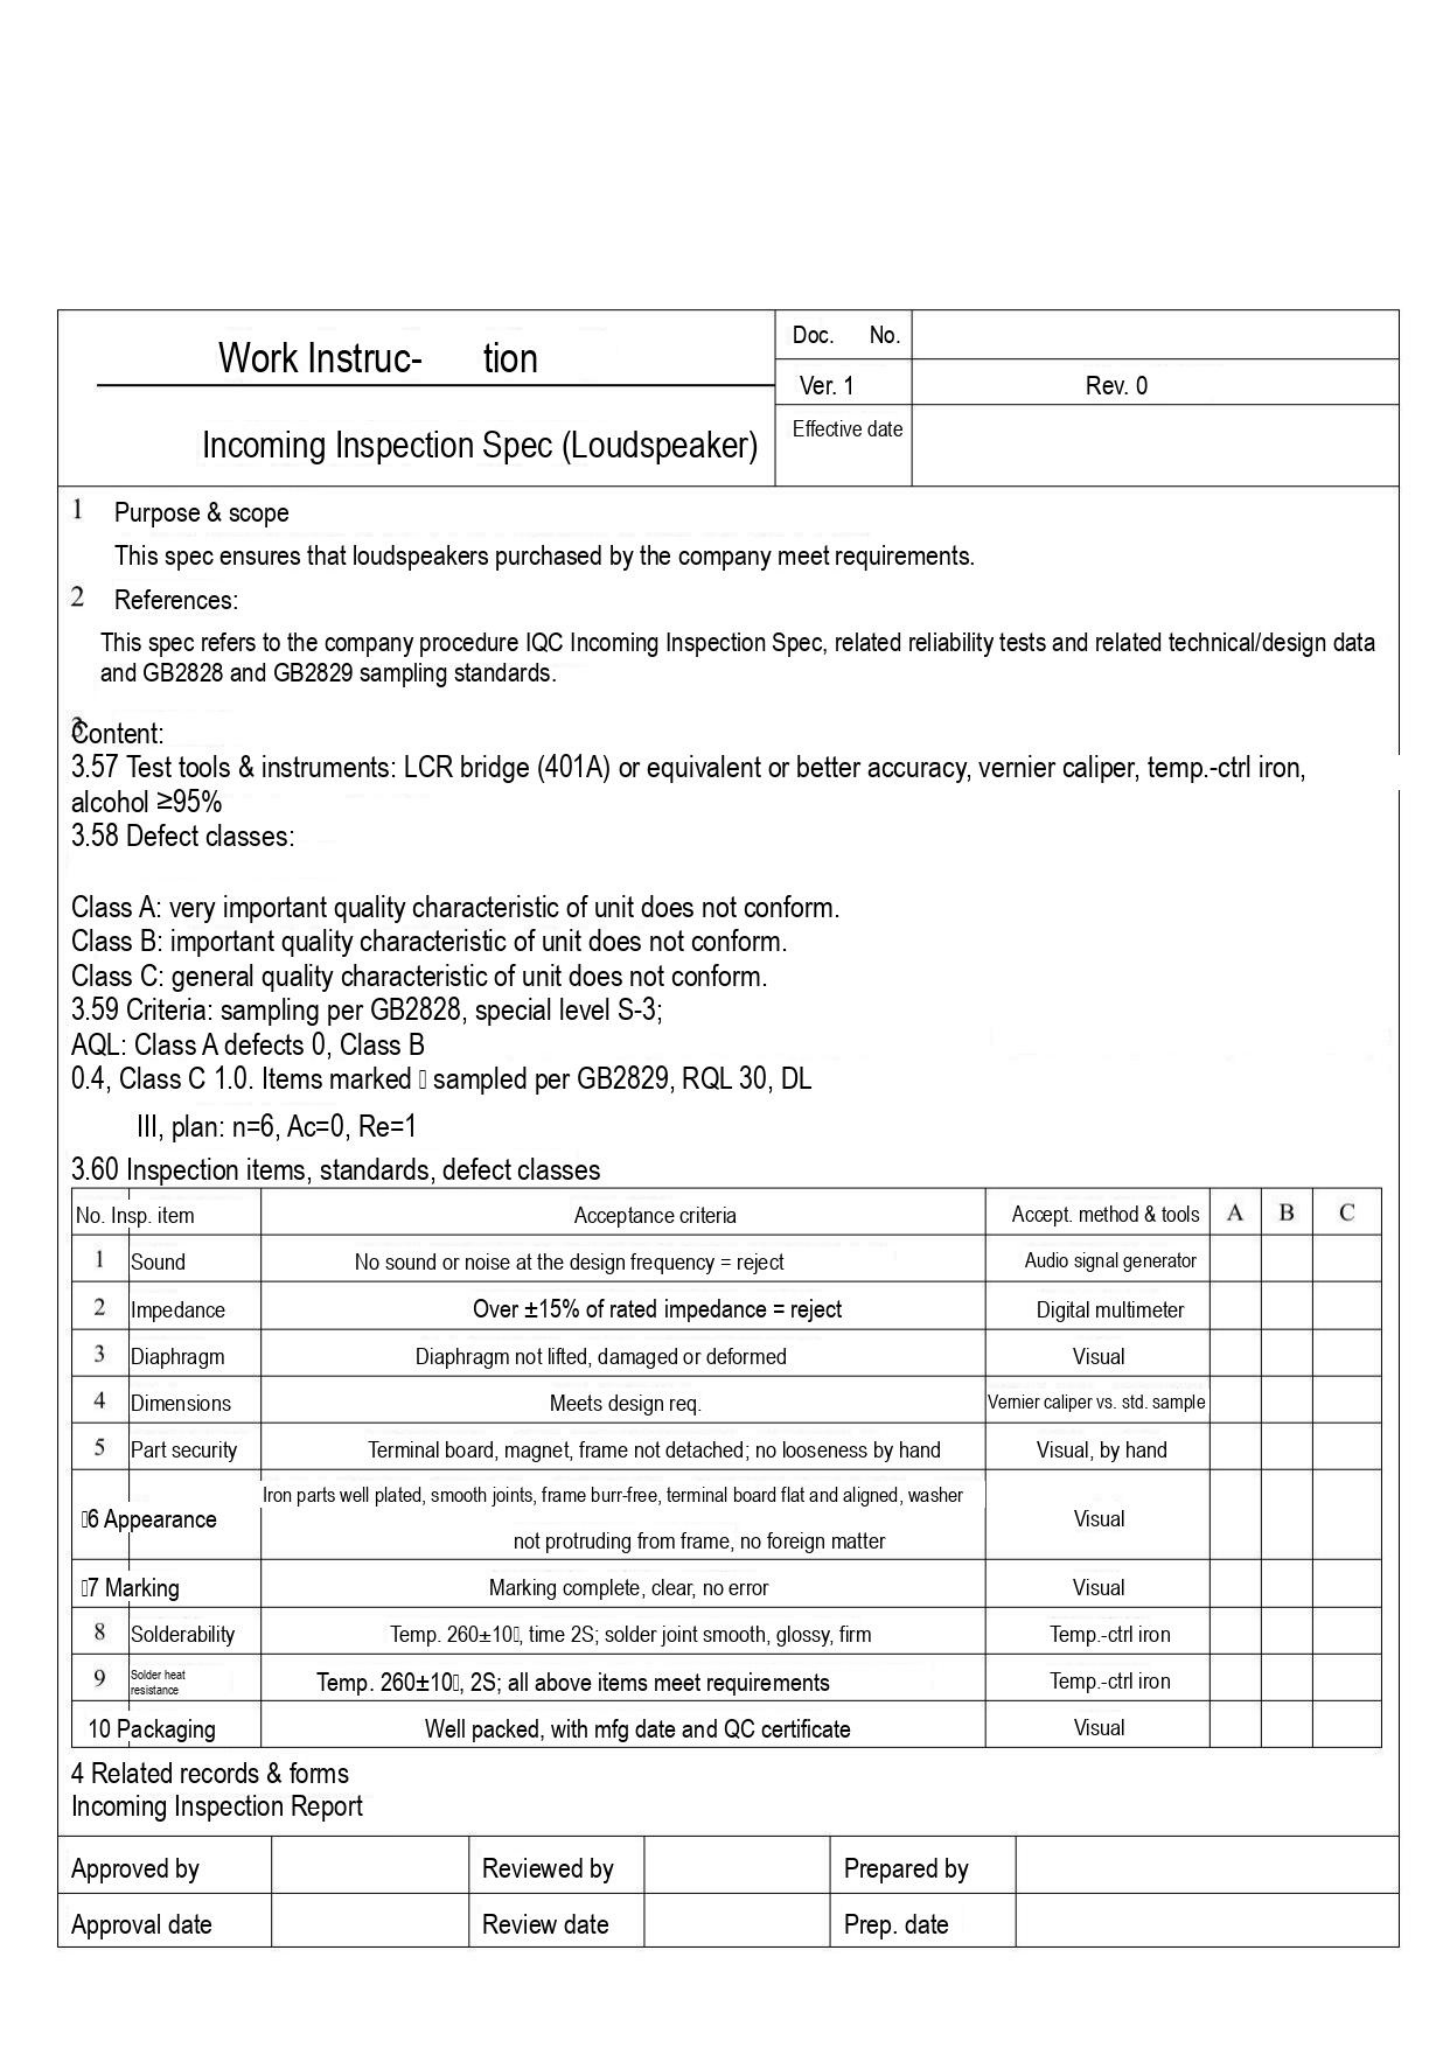| Work Instruc- tion | Doc. No. | |
|---|---|---|
| | Ver. 1 | Rev. 0 |
| Incoming Inspection Spec (Loudspeaker) | Effective date | |

1 Purpose & scope

This spec ensures that loudspeakers purchased by the company meet requirements.

2 References:

This spec refers to the company procedure IQC Incoming Inspection Spec, related reliability tests and related technical/design data and GB2828 and GB2829 sampling standards.

3 Content:

3.57 Test tools & instruments: LCR bridge (401A) or equivalent or better accuracy, vernier caliper, temp.-ctrl iron, alcohol ≥95%

3.58 Defect classes:

Class A: very important quality characteristic of unit does not conform.
Class B: important quality characteristic of unit does not conform.
Class C: general quality characteristic of unit does not conform.

3.59 Criteria: sampling per GB2828, special level S-3;
AQL: Class A defects 0, Class B
0.4, Class C 1.0. Items marked sampled per GB2829, RQL 30, DL
III, plan: n=6, Ac=0, Re=1

3.60 Inspection items, standards, defect classes

| No. | Insp. item | Acceptance criteria | Accept. method & tools | A | B | C |
|---|---|---|---|---|---|---|
| 1 | Sound | No sound or noise at the design frequency = reject | Audio signal generator | | | |
| 2 | Impedance | Over ±15% of rated impedance = reject | Digital multimeter | | | |
| 3 | Diaphragm | Diaphragm not lifted, damaged or deformed | Visual | | | |
| 4 | Dimensions | Meets design req. | Vernier caliper vs. std. sample | | | |
| 5 | Part security | Terminal board, magnet, frame not detached; no looseness by hand | Visual, by hand | | | |
| 6 | Appearance | Iron parts well plated, smooth joints, frame burr-free, terminal board flat and aligned, washer not protruding from frame, no foreign matter | Visual | | | |
| 7 | Marking | Marking complete, clear, no error | Visual | | | |
| 8 | Solderability | Temp. 260±10, time 2S; solder joint smooth, glossy, firm | Temp.-ctrl iron | | | |
| 9 | Solder heat resistance | Temp. 260±10, 2S; all above items meet requirements | Temp.-ctrl iron | | | |
| 10 | Packaging | Well packed, with mfg date and QC certificate | Visual | | | |

4 Related records & forms
Incoming Inspection Report

| Approved by | | Reviewed by | | Prepared by | |
|---|---|---|---|---|---|
| Approval date | | Review date | | Prep. date | |
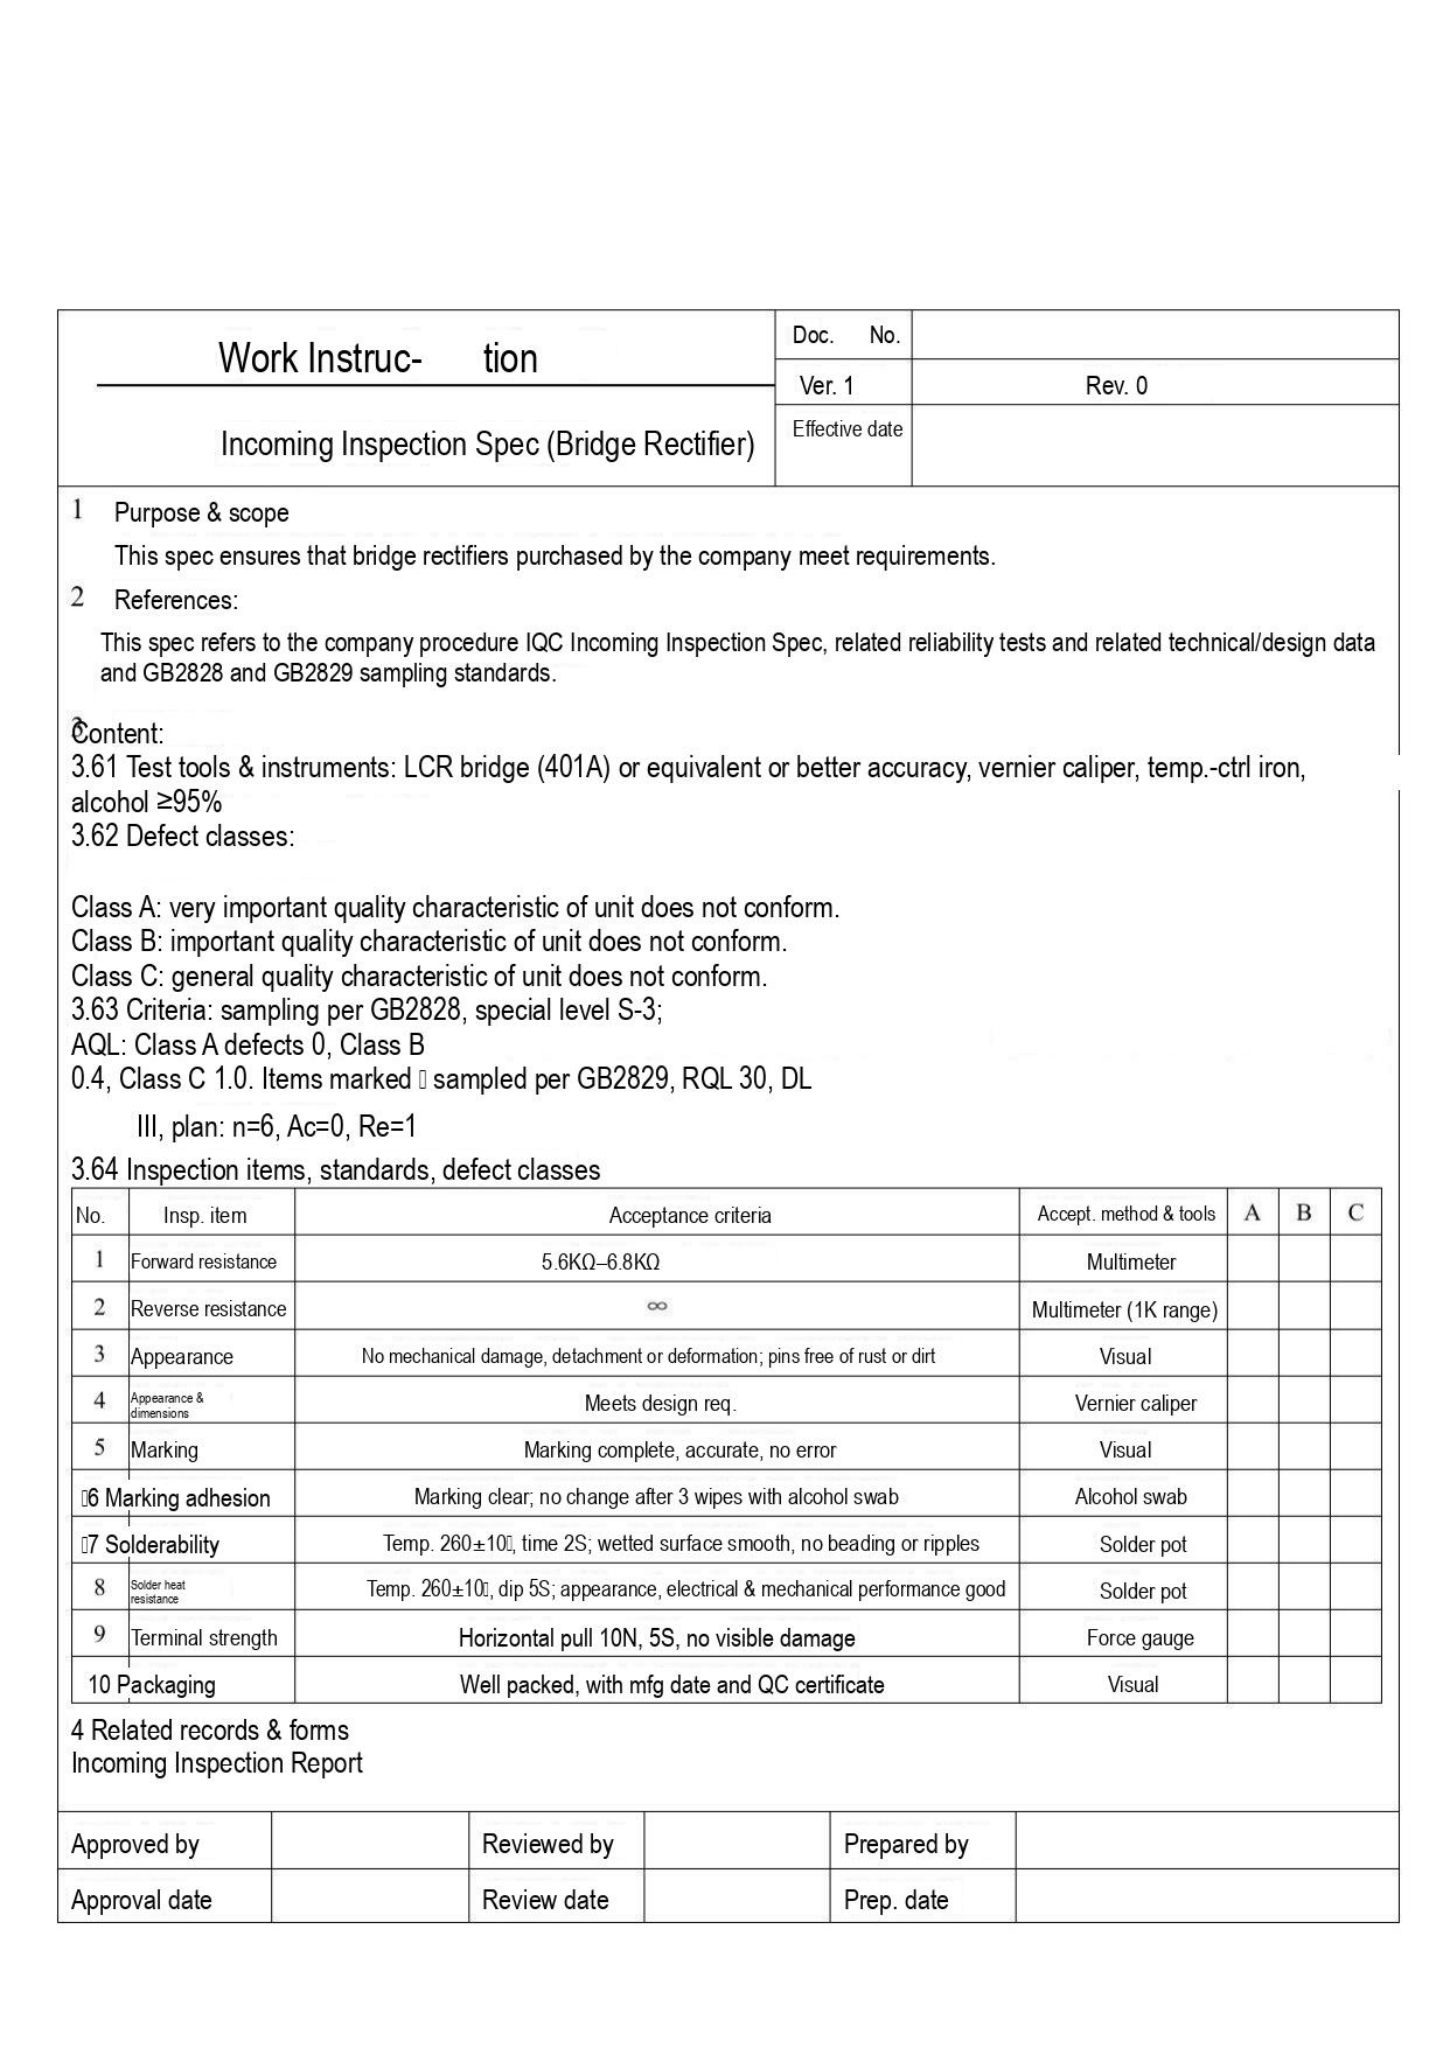| Work Instruc- tion | Doc. No. | |
|---|---|---|
| | Ver. 1 | Rev. 0 |
| Incoming Inspection Spec (Bridge Rectifier) | Effective date | |

1 Purpose & scope

This spec ensures that bridge rectifiers purchased by the company meet requirements.

2 References:

This spec refers to the company procedure IQC Incoming Inspection Spec, related reliability tests and related technical/design data and GB2828 and GB2829 sampling standards.

3 Content:
3.61 Test tools & instruments: LCR bridge (401A) or equivalent or better accuracy, vernier caliper, temp.-ctrl iron, alcohol ≥95%
3.62 Defect classes:

Class A: very important quality characteristic of unit does not conform.
Class B: important quality characteristic of unit does not conform.
Class C: general quality characteristic of unit does not conform.
3.63 Criteria: sampling per GB2828, special level S-3;
AQL: Class A defects 0, Class B
0.4, Class C 1.0. Items marked sampled per GB2829, RQL 30, DL

III, plan: n=6, Ac=0, Re=1

3.64 Inspection items, standards, defect classes

| No. | Insp. item | Acceptance criteria | Accept. method & tools | A | B | C |
|---|---|---|---|---|---|---|
| 1 | Forward resistance | 5.6KΩ–6.8KΩ | Multimeter | | | |
| 2 | Reverse resistance | ∞ | Multimeter (1K range) | | | |
| 3 | Appearance | No mechanical damage, detachment or deformation; pins free of rust or dirt | Visual | | | |
| 4 | Appearance & dimensions | Meets design req. | Vernier caliper | | | |
| 5 | Marking | Marking complete, accurate, no error | Visual | | | |
| 6 | Marking adhesion | Marking clear; no change after 3 wipes with alcohol swab | Alcohol swab | | | |
| 7 | Solderability | Temp. 260±10, time 2S; wetted surface smooth, no beading or ripples | Solder pot | | | |
| 8 | Solder heat resistance | Temp. 260±10, dip 5S; appearance, electrical & mechanical performance good | Solder pot | | | |
| 9 | Terminal strength | Horizontal pull 10N, 5S, no visible damage | Force gauge | | | |
| 10 | Packaging | Well packed, with mfg date and QC certificate | Visual | | | |

4 Related records & forms
Incoming Inspection Report

| Approved by | | Reviewed by | | Prepared by | |
|---|---|---|---|---|---|
| Approval date | | Review date | | Prep. date | |
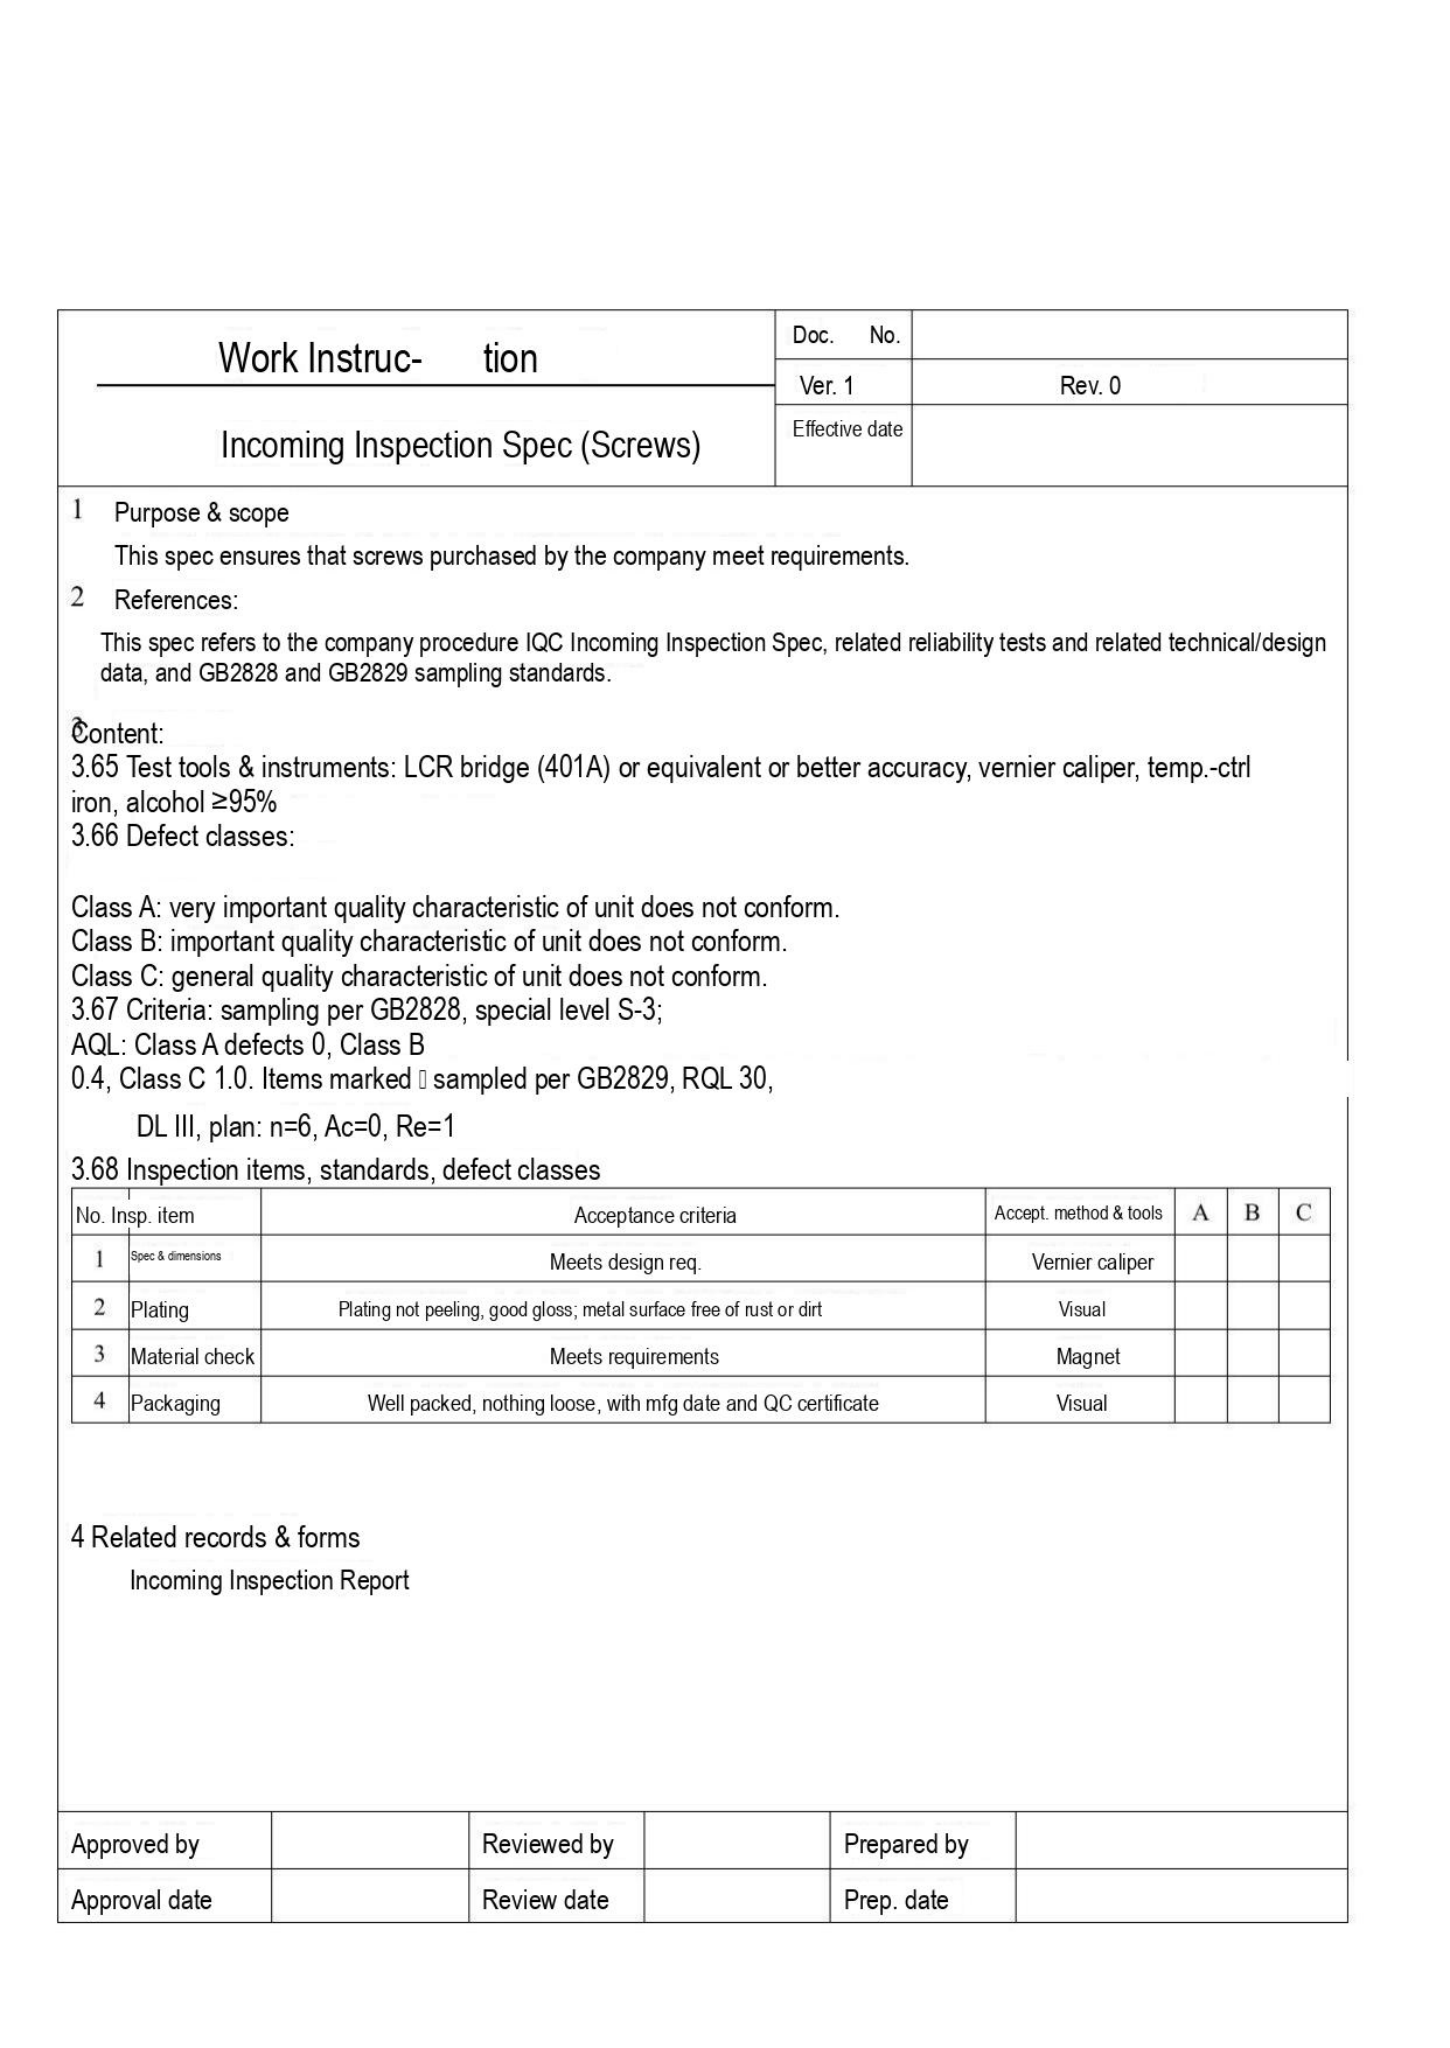| Work Instruc- tion | Doc. No. | |
|---|---|---|
| | Ver. 1 | Rev. 0 |
| Incoming Inspection Spec (Screws) | Effective date | |

1 Purpose & scope

This spec ensures that screws purchased by the company meet requirements.

2 References:

This spec refers to the company procedure IQC Incoming Inspection Spec, related reliability tests and related technical/design data, and GB2828 and GB2829 sampling standards.

3 Content:

3.65 Test tools & instruments: LCR bridge (401A) or equivalent or better accuracy, vernier caliper, temp.-ctrl iron, alcohol ≥95%

3.66 Defect classes:

Class A: very important quality characteristic of unit does not conform.
Class B: important quality characteristic of unit does not conform.
Class C: general quality characteristic of unit does not conform.

3.67 Criteria: sampling per GB2828, special level S-3;
AQL: Class A defects 0, Class B
0.4, Class C 1.0. Items marked sampled per GB2829, RQL 30,

DL III, plan: n=6, Ac=0, Re=1

3.68 Inspection items, standards, defect classes

| No. | Insp. item | Acceptance criteria | Accept. method & tools | A | B | C |
|---|---|---|---|---|---|---|
| 1 | Spec & dimensions | Meets design req. | Vernier caliper | | | |
| 2 | Plating | Plating not peeling, good gloss; metal surface free of rust or dirt | Visual | | | |
| 3 | Material check | Meets requirements | Magnet | | | |
| 4 | Packaging | Well packed, nothing loose, with mfg date and QC certificate | Visual | | | |

4 Related records & forms

Incoming Inspection Report

| Approved by | | Reviewed by | | Prepared by | |
|---|---|---|---|---|---|
| Approval date | | Review date | | Prep. date | |
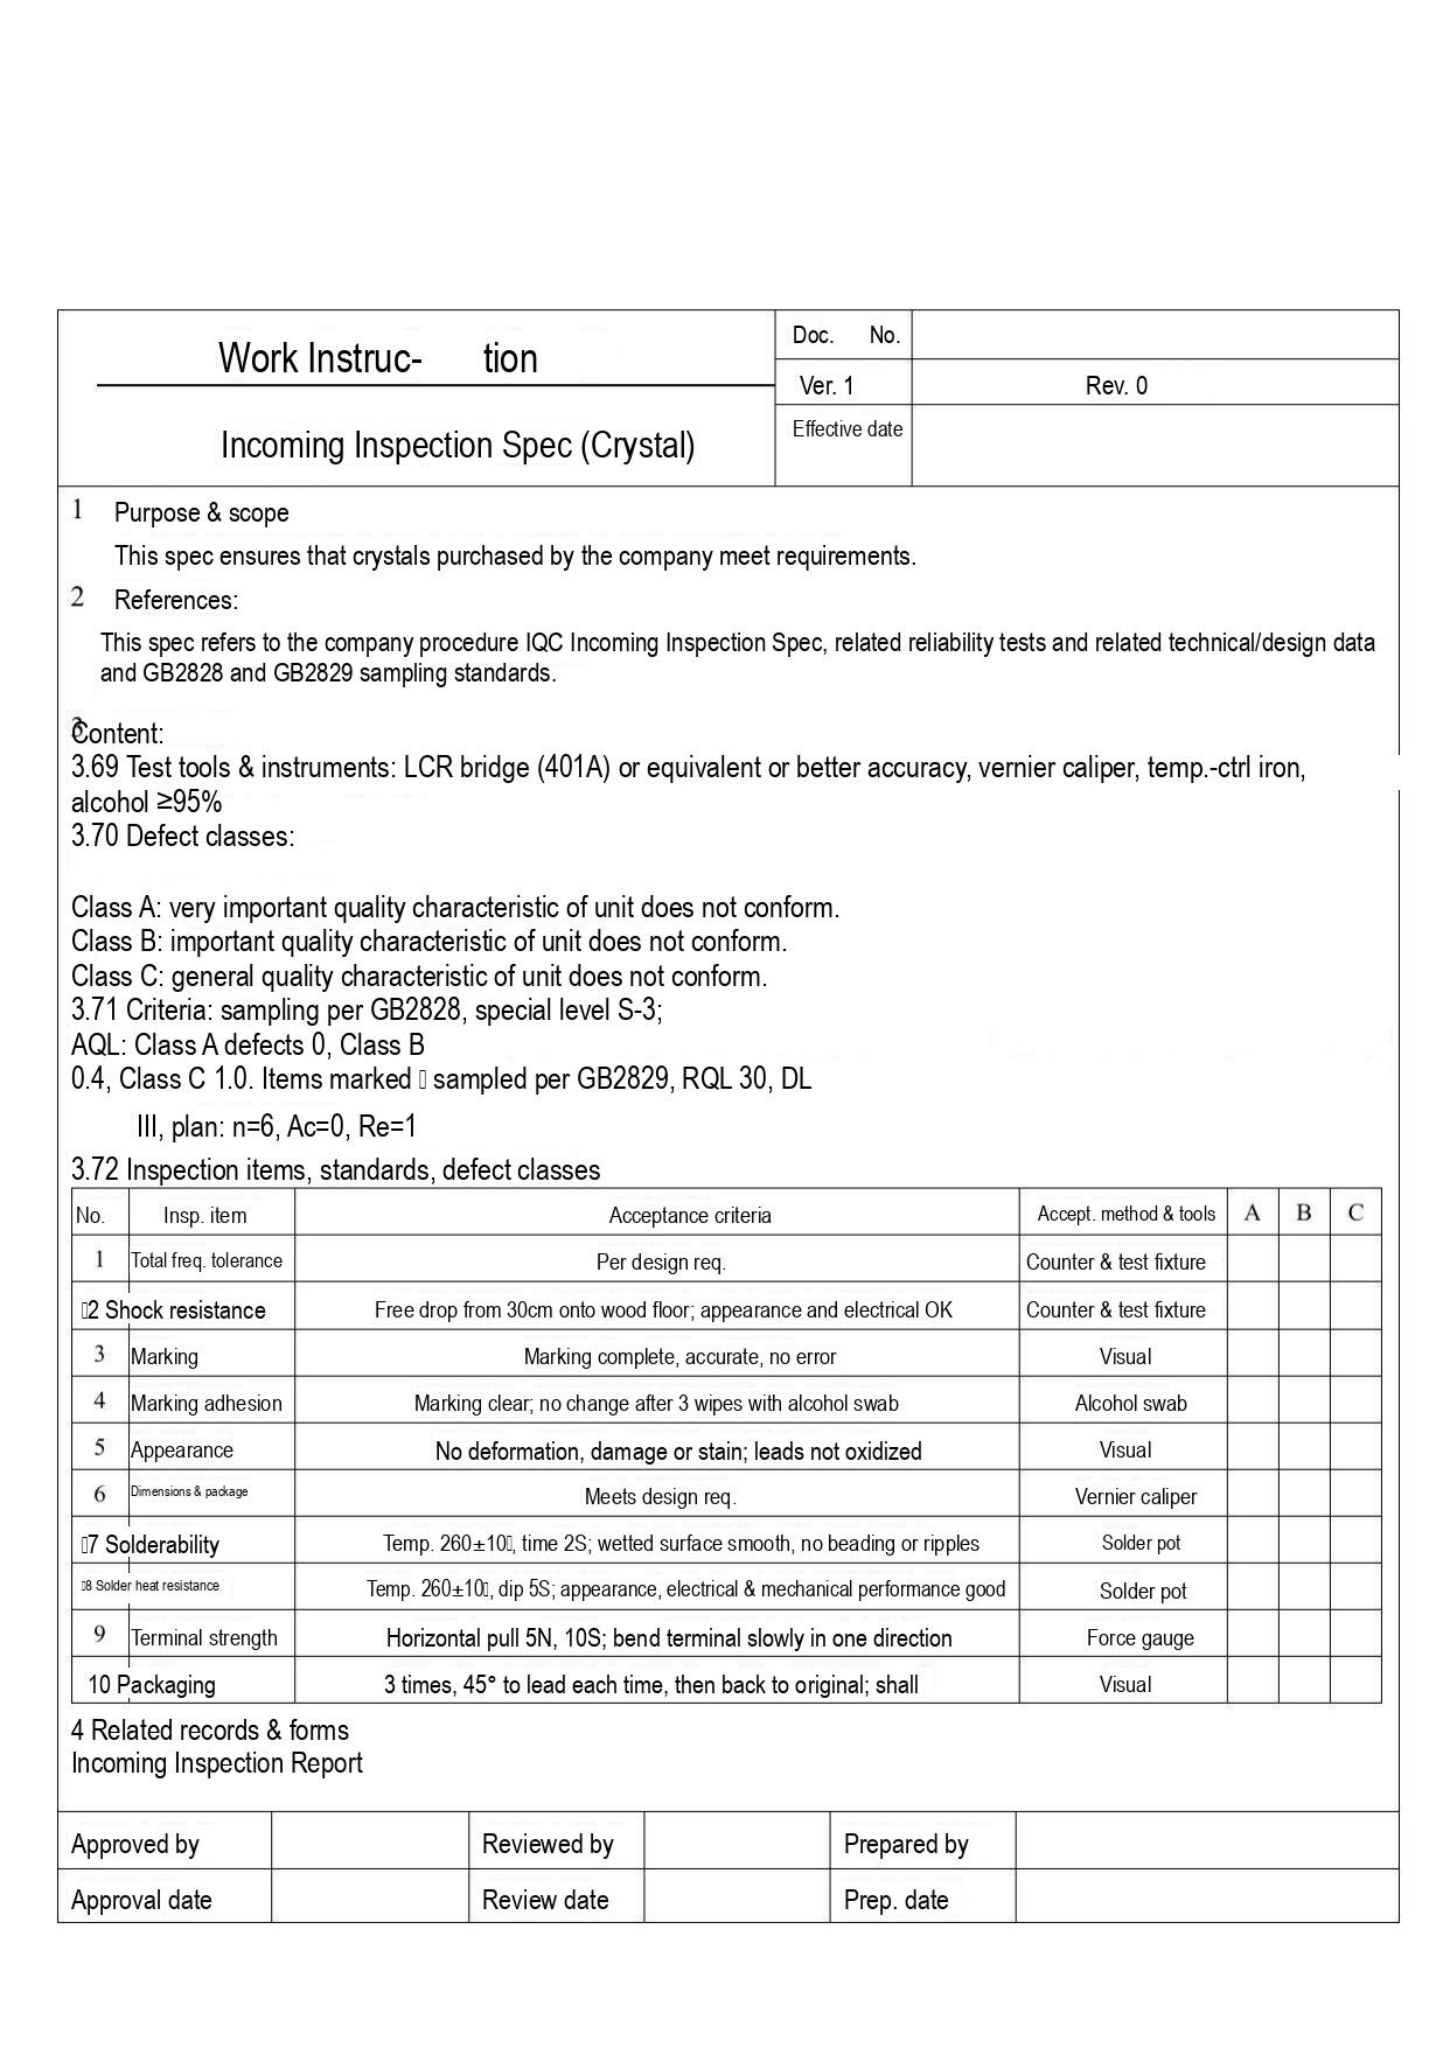| Work Instruc- tion | Doc. No. | |
|---|---|---|
| | Ver. 1 | Rev. 0 |
| Incoming Inspection Spec (Crystal) | Effective date | |

1 Purpose & scope

This spec ensures that crystals purchased by the company meet requirements.

2 References:

This spec refers to the company procedure IQC Incoming Inspection Spec, related reliability tests and related technical/design data and GB2828 and GB2829 sampling standards.

3 Content:

3.69 Test tools & instruments: LCR bridge (401A) or equivalent or better accuracy, vernier caliper, temp.-ctrl iron, alcohol ≥95%

3.70 Defect classes:

Class A: very important quality characteristic of unit does not conform.
Class B: important quality characteristic of unit does not conform.
Class C: general quality characteristic of unit does not conform.

3.71 Criteria: sampling per GB2828, special level S-3;
AQL: Class A defects 0, Class B
0.4, Class C 1.0. Items marked sampled per GB2829, RQL 30, DL
III, plan: n=6, Ac=0, Re=1

3.72 Inspection items, standards, defect classes

| No. | Insp. item | Acceptance criteria | Accept. method & tools | A | B | C |
|---|---|---|---|---|---|---|
| 1 | Total freq. tolerance | Per design req. | Counter & test fixture | | | |
| 2 | Shock resistance | Free drop from 30cm onto wood floor; appearance and electrical OK | Counter & test fixture | | | |
| 3 | Marking | Marking complete, accurate, no error | Visual | | | |
| 4 | Marking adhesion | Marking clear; no change after 3 wipes with alcohol swab | Alcohol swab | | | |
| 5 | Appearance | No deformation, damage or stain; leads not oxidized | Visual | | | |
| 6 | Dimensions & package | Meets design req. | Vernier caliper | | | |
| 7 | Solderability | Temp. 260±10, time 2S; wetted surface smooth, no beading or ripples | Solder pot | | | |
| 8 | Solder heat resistance | Temp. 260±10, dip 5S; appearance, electrical & mechanical performance good | Solder pot | | | |
| 9 | Terminal strength | Horizontal pull 5N, 10S; bend terminal slowly in one direction | Force gauge | | | |
| 10 | Packaging | 3 times, 45° to lead each time, then back to original; shall | Visual | | | |

4 Related records & forms
Incoming Inspection Report

| Approved by | | Reviewed by | | Prepared by | |
|---|---|---|---|---|---|
| Approval date | | Review date | | Prep. date | |
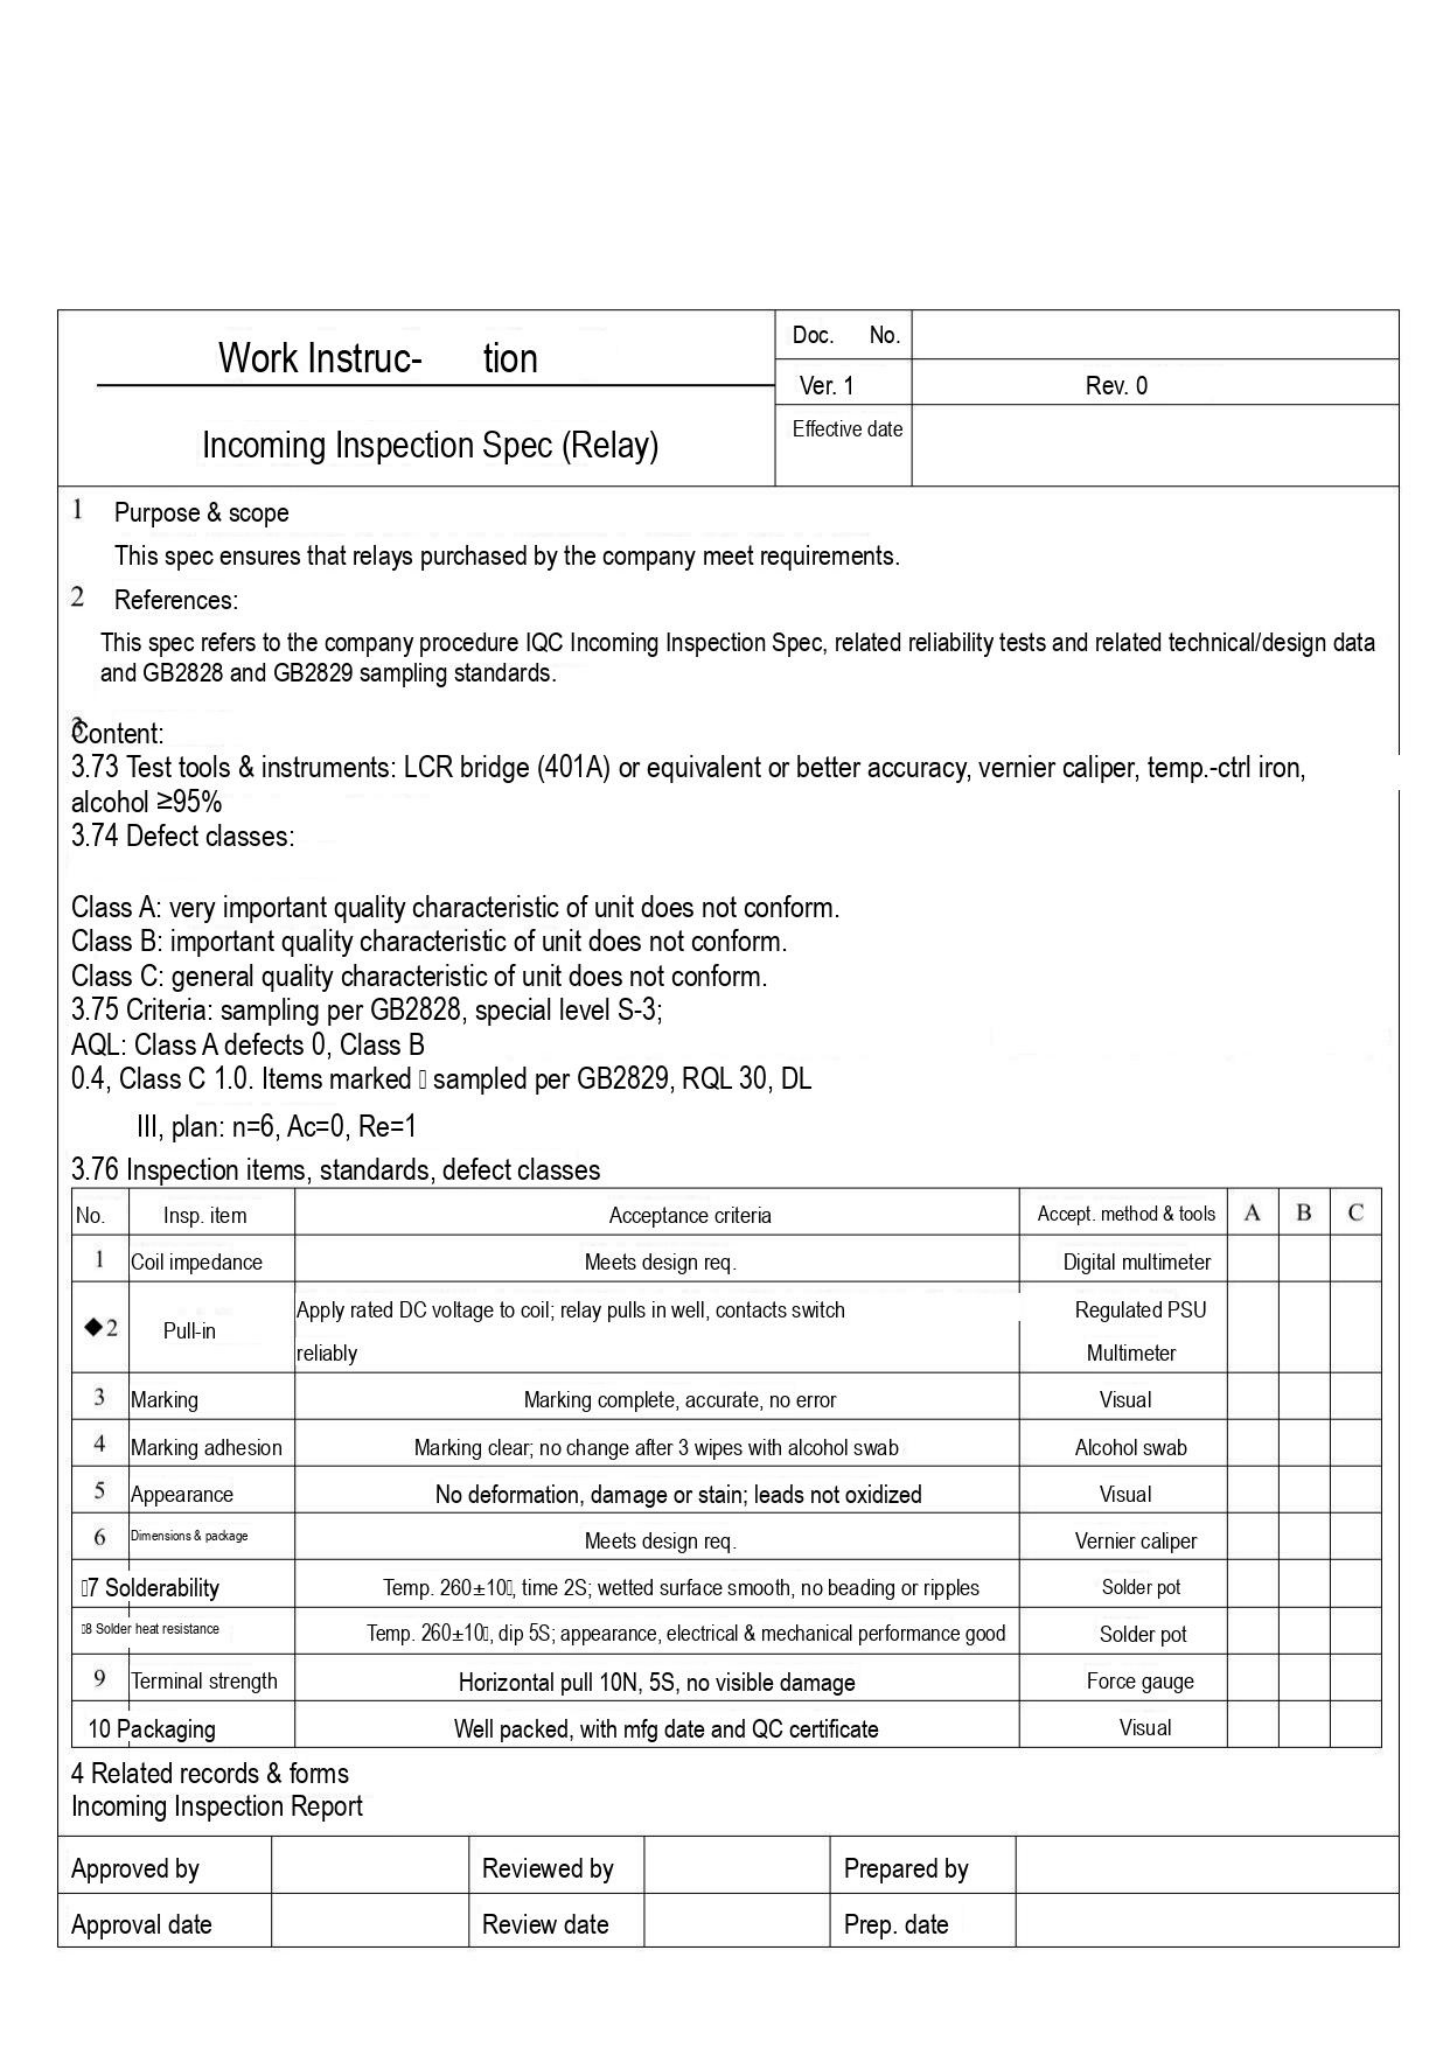| Work Instruc- tion | Doc. No. | |
|---|---|---|
| | Ver. 1 | Rev. 0 |
| Incoming Inspection Spec (Relay) | Effective date | |

1 Purpose & scope

This spec ensures that relays purchased by the company meet requirements.

2 References:

This spec refers to the company procedure IQC Incoming Inspection Spec, related reliability tests and related technical/design data and GB2828 and GB2829 sampling standards.

Content:

3.73 Test tools & instruments: LCR bridge (401A) or equivalent or better accuracy, vernier caliper, temp.-ctrl iron, alcohol ≥95%

3.74 Defect classes:

Class A: very important quality characteristic of unit does not conform.
Class B: important quality characteristic of unit does not conform.
Class C: general quality characteristic of unit does not conform.

3.75 Criteria: sampling per GB2828, special level S-3;
AQL: Class A defects 0, Class B 0.4, Class C 1.0. Items marked sampled per GB2829, RQL 30, DL III, plan: n=6, Ac=0, Re=1

3.76 Inspection items, standards, defect classes

| No. | Insp. item | Acceptance criteria | Accept. method & tools | A | B | C |
|---|---|---|---|---|---|---|
| 1 | Coil impedance | Meets design req. | Digital multimeter | | | |
| ◆2 | Pull-in | Apply rated DC voltage to coil; relay pulls in well, contacts switch reliably | Regulated PSU Multimeter | | | |
| 3 | Marking | Marking complete, accurate, no error | Visual | | | |
| 4 | Marking adhesion | Marking clear; no change after 3 wipes with alcohol swab | Alcohol swab | | | |
| 5 | Appearance | No deformation, damage or stain; leads not oxidized | Visual | | | |
| 6 | Dimensions & package | Meets design req. | Vernier caliper | | | |
| 7 | Solderability | Temp. 260±10, time 2S; wetted surface smooth, no beading or ripples | Solder pot | | | |
| 8 | Solder heat resistance | Temp. 260±10, dip 5S; appearance, electrical & mechanical performance good | Solder pot | | | |
| 9 | Terminal strength | Horizontal pull 10N, 5S, no visible damage | Force gauge | | | |
| 10 | Packaging | Well packed, with mfg date and QC certificate | Visual | | | |

4 Related records & forms

Incoming Inspection Report

| Approved by | | Reviewed by | | Prepared by | |
|---|---|---|---|---|---|
| Approval date | | Review date | | Prep. date | |
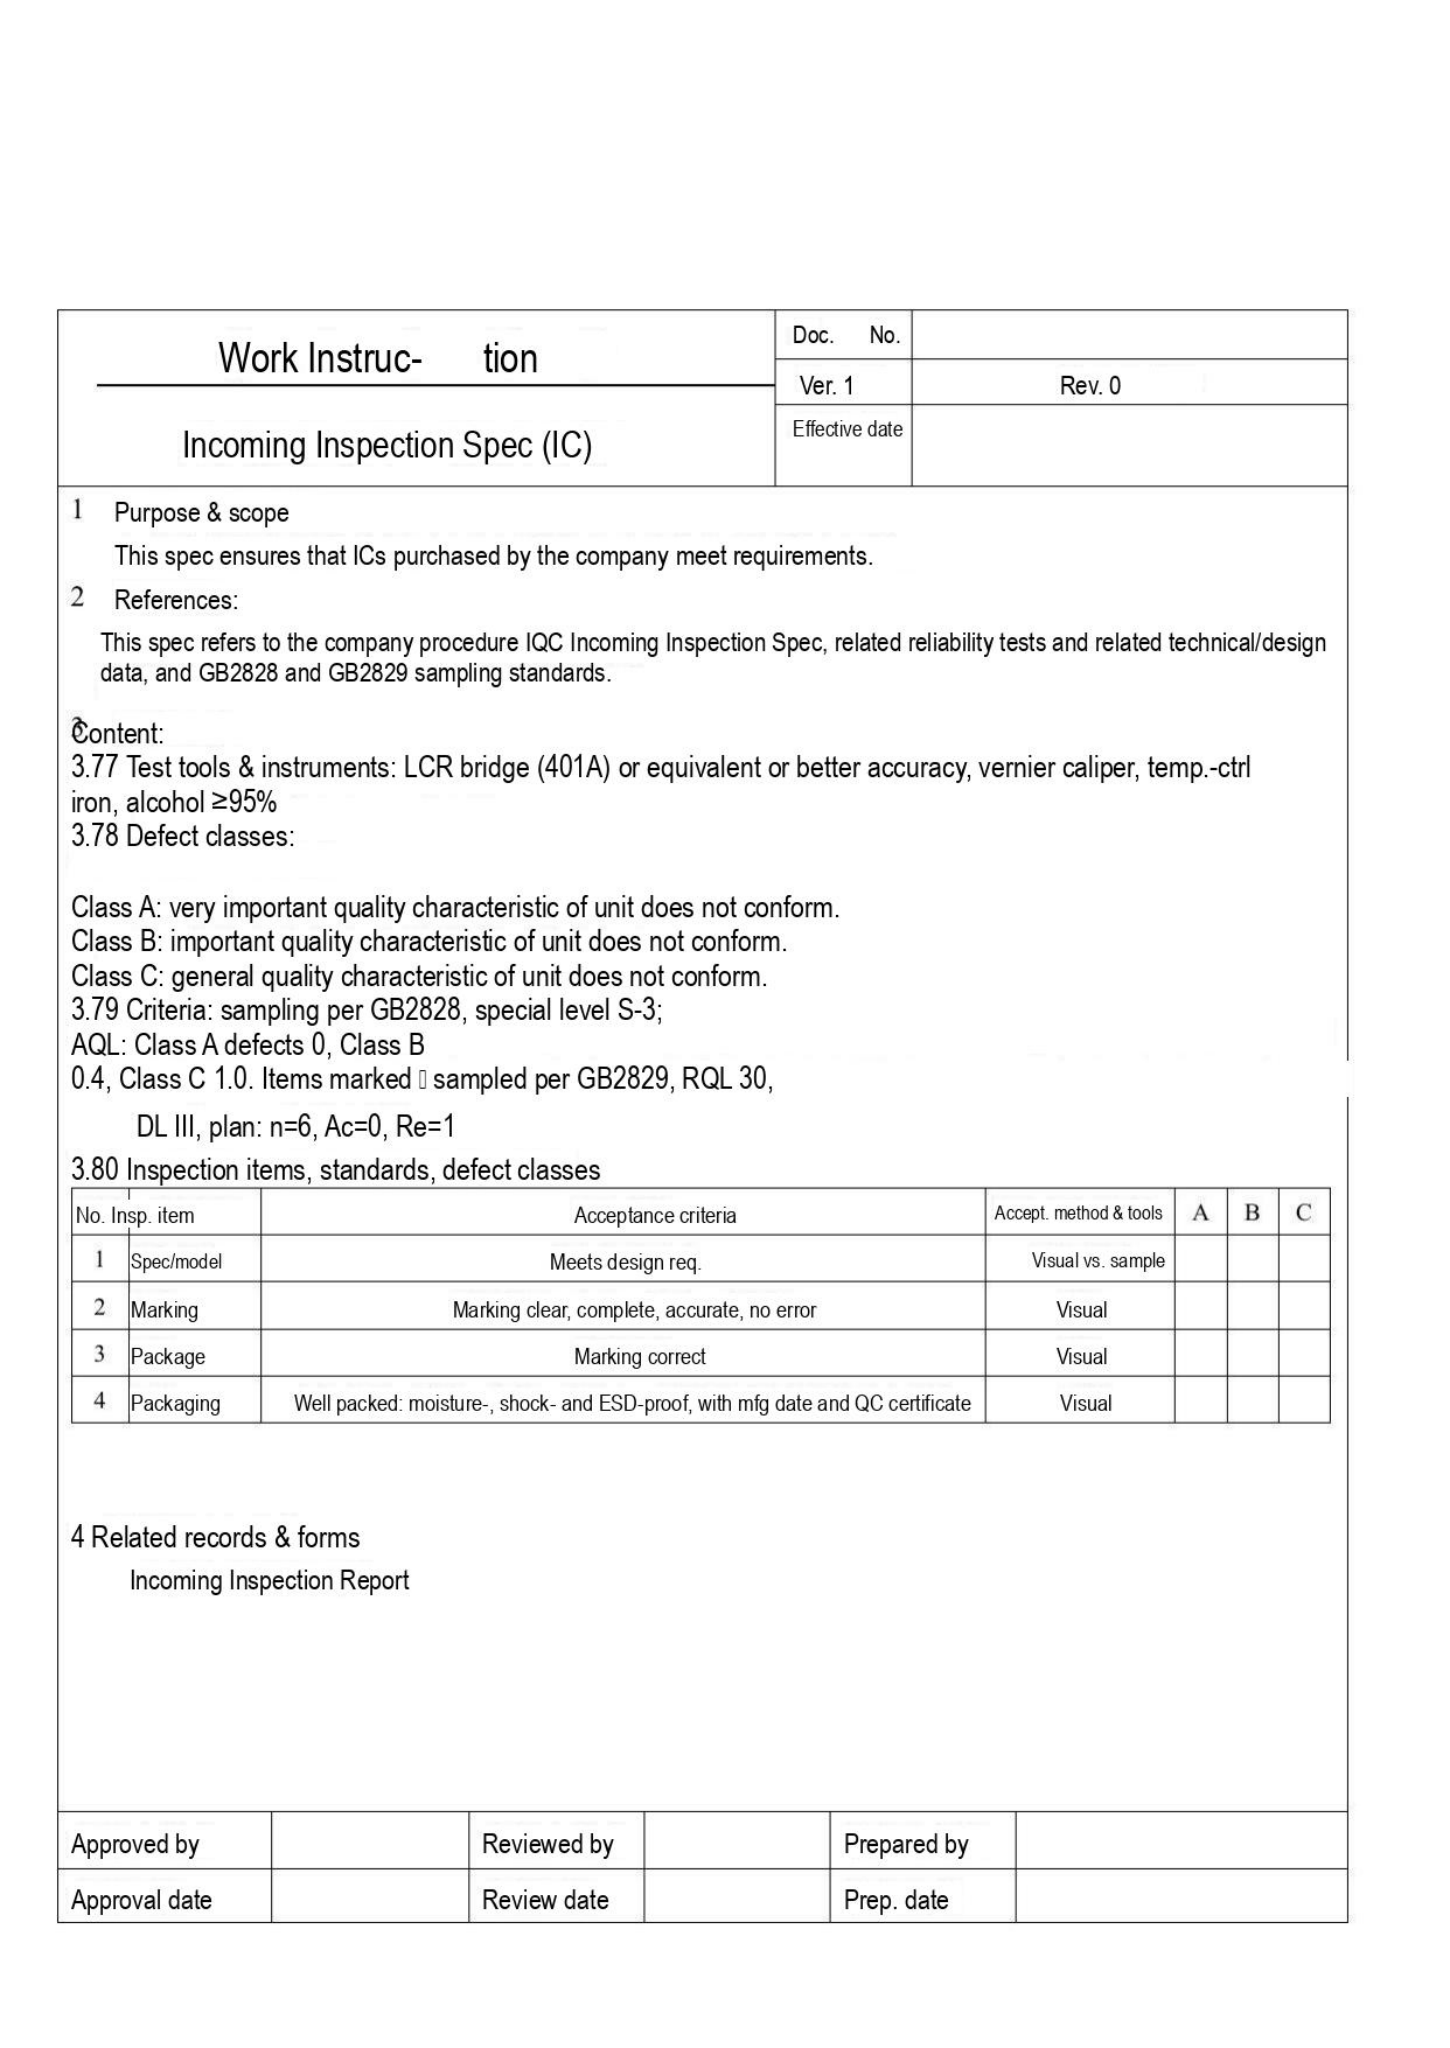| Work Instruc- tion | Doc. No. | |
|---|---|---|
| | Ver. 1 | Rev. 0 |
| Incoming Inspection Spec (IC) | Effective date | |

1 Purpose & scope

This spec ensures that ICs purchased by the company meet requirements.

2 References:

This spec refers to the company procedure IQC Incoming Inspection Spec, related reliability tests and related technical/design data, and GB2828 and GB2829 sampling standards.

3 Content:

3.77 Test tools & instruments: LCR bridge (401A) or equivalent or better accuracy, vernier caliper, temp.-ctrl iron, alcohol ≥95%

3.78 Defect classes:

Class A: very important quality characteristic of unit does not conform.
Class B: important quality characteristic of unit does not conform.
Class C: general quality characteristic of unit does not conform.

3.79 Criteria: sampling per GB2828, special level S-3;
AQL: Class A defects 0, Class B
0.4, Class C 1.0. Items marked sampled per GB2829, RQL 30,

DL III, plan: n=6, Ac=0, Re=1

3.80 Inspection items, standards, defect classes

| No. | Insp. item | Acceptance criteria | Accept. method & tools | A | B | C |
|---|---|---|---|---|---|---|
| 1 | Spec/model | Meets design req. | Visual vs. sample | | | |
| 2 | Marking | Marking clear, complete, accurate, no error | Visual | | | |
| 3 | Package | Marking correct | Visual | | | |
| 4 | Packaging | Well packed: moisture-, shock- and ESD-proof, with mfg date and QC certificate | Visual | | | |

4 Related records & forms

Incoming Inspection Report

| Approved by | | Reviewed by | | Prepared by | |
|---|---|---|---|---|---|
| Approval date | | Review date | | Prep. date | |